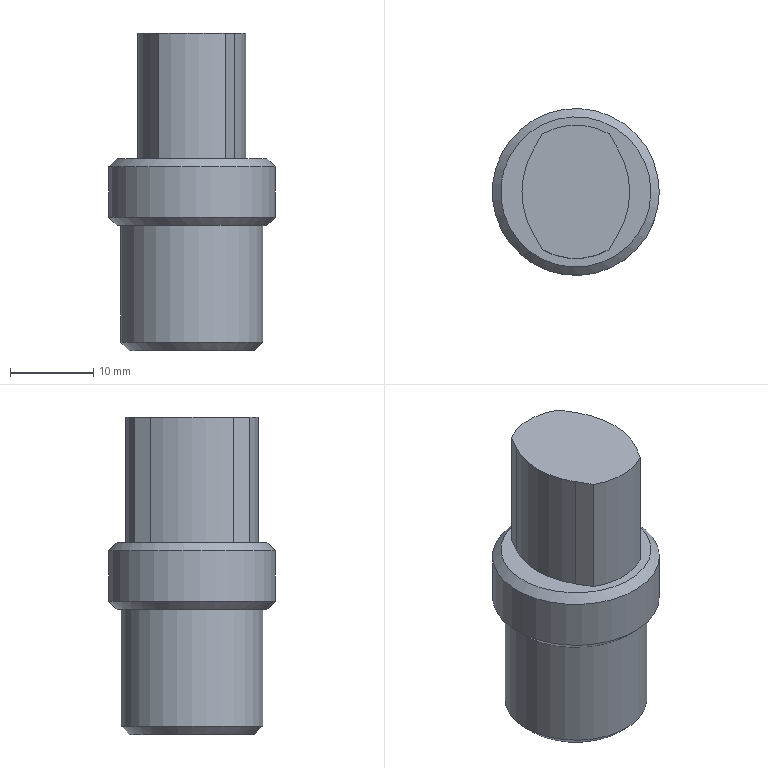Part | NX | features DATUM_CSYS 4, EXTRUDE 3, SKETCH 3, BLEND 1, CHAMFER 1 | 1 solid | 17 faces | box 20 x 20 x 38 mm | volume 8338 mm3 | plane 8 | cylinder 6 | cone 3 | commonest cylinder face diameters 20 x3 16 x2 17 x1
STEP:
#1=CARTESIAN_POINT('',(8.5,0.,1.));
#2=VERTEX_POINT('',#1);
#3=CARTESIAN_POINT('',(0.,0.,1.));
#4=DIRECTION('',(0.,0.,1.));
#5=DIRECTION('',(1.,0.,0.));
#6=AXIS2_PLACEMENT_3D('',#3,#4,#5);
#7=CIRCLE('',#6,8.5);
#8=EDGE_CURVE('',#2,#2,#7,.T.);
#9=ORIENTED_EDGE('',*,*,#8,.T.);
#10=EDGE_LOOP('',(#9));
#11=FACE_BOUND('',#10,.T.);
#12=CARTESIAN_POINT('',(8.5,0.,15.));
#13=VERTEX_POINT('',#12);
#14=CARTESIAN_POINT('',(0.,0.,15.));
#15=DIRECTION('',(0.,0.,1.));
#16=DIRECTION('',(1.,0.,0.));
#17=AXIS2_PLACEMENT_3D('',#14,#15,#16);
#18=CIRCLE('',#17,8.5);
#19=EDGE_CURVE('',#13,#13,#18,.T.);
#20=ORIENTED_EDGE('',*,*,#19,.F.);
#21=EDGE_LOOP('',(#20));
#22=FACE_BOUND('',#21,.T.);
#23=CARTESIAN_POINT('',(0.,0.,15.));
#24=DIRECTION('',(0.,0.,-1.));
#25=DIRECTION('',(-1.,0.,0.));
#26=AXIS2_PLACEMENT_3D('',#23,#24,#25);
#27=CYLINDRICAL_SURFACE('',#26,8.5);
#28=ADVANCED_FACE('',(#11,#22),#27,.T.);
#29=CARTESIAN_POINT('',(7.5,0.,0.));
#30=VERTEX_POINT('',#29);
#31=CARTESIAN_POINT('',(0.,0.,0.));
#32=DIRECTION('',(0.,0.,1.));
#33=DIRECTION('',(1.,0.,0.));
#34=AXIS2_PLACEMENT_3D('',#31,#32,#33);
#35=CIRCLE('',#34,7.5);
#36=EDGE_CURVE('',#30,#30,#35,.F.);
#37=ORIENTED_EDGE('',*,*,#36,.T.);
#38=EDGE_LOOP('',(#37));
#39=FACE_BOUND('',#38,.T.);
#40=CARTESIAN_POINT('',(0.,0.,0.));
#41=DIRECTION('',(0.,0.,1.));
#42=DIRECTION('',(1.,0.,0.));
#43=AXIS2_PLACEMENT_3D('',#40,#41,#42);
#44=PLANE('',#43);
#45=ADVANCED_FACE('',(#39),#44,.F.);
#46=CARTESIAN_POINT('',(10.,0.,22.));
#47=VERTEX_POINT('',#46);
#48=CARTESIAN_POINT('',(0.,0.,22.));
#49=DIRECTION('',(0.,0.,1.));
#50=DIRECTION('',(1.,0.,0.));
#51=AXIS2_PLACEMENT_3D('',#48,#49,#50);
#52=CIRCLE('',#51,10.);
#53=EDGE_CURVE('',#47,#47,#52,.F.);
#54=ORIENTED_EDGE('',*,*,#53,.T.);
#55=EDGE_LOOP('',(#54));
#56=FACE_BOUND('',#55,.T.);
#57=CARTESIAN_POINT('',(10.,0.,16.));
#58=VERTEX_POINT('',#57);
#59=CARTESIAN_POINT('',(0.,0.,16.));
#60=DIRECTION('',(0.,0.,1.));
#61=DIRECTION('',(1.,0.,0.));
#62=AXIS2_PLACEMENT_3D('',#59,#60,#61);
#63=CIRCLE('',#62,10.);
#64=EDGE_CURVE('',#58,#58,#63,.T.);
#65=ORIENTED_EDGE('',*,*,#64,.T.);
#66=EDGE_LOOP('',(#65));
#67=FACE_BOUND('',#66,.T.);
#68=CARTESIAN_POINT('',(0.,0.,23.));
#69=DIRECTION('',(0.,0.,-1.));
#70=DIRECTION('',(-1.,0.,0.));
#71=AXIS2_PLACEMENT_3D('',#68,#69,#70);
#72=CYLINDRICAL_SURFACE('',#71,10.);
#73=ADVANCED_FACE('',(#56,#67),#72,.T.);
#74=CARTESIAN_POINT('',(9.,0.,23.));
#75=VERTEX_POINT('',#74);
#76=CARTESIAN_POINT('',(0.,0.,23.));
#77=DIRECTION('',(0.,0.,1.));
#78=DIRECTION('',(1.,0.,0.));
#79=AXIS2_PLACEMENT_3D('',#76,#77,#78);
#80=CIRCLE('',#79,9.);
#81=EDGE_CURVE('',#75,#75,#80,.T.);
#82=ORIENTED_EDGE('',*,*,#81,.T.);
#83=EDGE_LOOP('',(#82));
#84=FACE_BOUND('',#83,.T.);
#85=CARTESIAN_POINT('',(5.113,5.,23.));
#86=VERTEX_POINT('',#85);
#87=CARTESIAN_POINT('',(4.,6.928,23.));
#88=VERTEX_POINT('',#87);
#89=CARTESIAN_POINT('',(8.,0.,23.));
#90=DIRECTION('',(-0.5,0.866,0.));
#91=VECTOR('',#90,1000.);
#92=LINE('',#89,#91);
#93=EDGE_CURVE('',#86,#88,#92,.T.);
#94=ORIENTED_EDGE('',*,*,#93,.F.);
#95=CARTESIAN_POINT('',(5.113,-5.,23.));
#96=VERTEX_POINT('',#95);
#97=CARTESIAN_POINT('',(-3.547,0.,23.));
#98=DIRECTION('',(0.,0.,1.));
#99=DIRECTION('',(1.,0.,0.));
#100=AXIS2_PLACEMENT_3D('',#97,#98,#99);
#101=CIRCLE('',#100,10.);
#102=EDGE_CURVE('',#86,#96,#101,.F.);
#103=ORIENTED_EDGE('',*,*,#102,.T.);
#104=CARTESIAN_POINT('',(4.,-6.928,23.));
#105=VERTEX_POINT('',#104);
#106=CARTESIAN_POINT('',(4.,-6.928,23.));
#107=DIRECTION('',(0.5,0.866,0.));
#108=VECTOR('',#107,1000.);
#109=LINE('',#106,#108);
#110=EDGE_CURVE('',#105,#96,#109,.T.);
#111=ORIENTED_EDGE('',*,*,#110,.F.);
#112=CARTESIAN_POINT('',(-4.,-6.928,23.));
#113=VERTEX_POINT('',#112);
#114=CARTESIAN_POINT('',(0.,0.,23.));
#115=DIRECTION('',(0.,0.,1.));
#116=DIRECTION('',(1.,0.,0.));
#117=AXIS2_PLACEMENT_3D('',#114,#115,#116);
#118=CIRCLE('',#117,8.);
#119=EDGE_CURVE('',#113,#105,#118,.T.);
#120=ORIENTED_EDGE('',*,*,#119,.F.);
#121=CARTESIAN_POINT('',(-5.113,-5.,23.));
#122=VERTEX_POINT('',#121);
#123=CARTESIAN_POINT('',(-8.,0.,23.));
#124=DIRECTION('',(0.5,-0.866,0.));
#125=VECTOR('',#124,1000.);
#126=LINE('',#123,#125);
#127=EDGE_CURVE('',#122,#113,#126,.T.);
#128=ORIENTED_EDGE('',*,*,#127,.F.);
#129=CARTESIAN_POINT('',(-5.113,5.,23.));
#130=VERTEX_POINT('',#129);
#131=CARTESIAN_POINT('',(3.547,0.,23.));
#132=DIRECTION('',(0.,0.,1.));
#133=DIRECTION('',(1.,0.,0.));
#134=AXIS2_PLACEMENT_3D('',#131,#132,#133);
#135=CIRCLE('',#134,10.);
#136=EDGE_CURVE('',#122,#130,#135,.F.);
#137=ORIENTED_EDGE('',*,*,#136,.T.);
#138=CARTESIAN_POINT('',(-4.,6.928,23.));
#139=VERTEX_POINT('',#138);
#140=CARTESIAN_POINT('',(-4.,6.928,23.));
#141=DIRECTION('',(-0.5,-0.866,0.));
#142=VECTOR('',#141,1000.);
#143=LINE('',#140,#142);
#144=EDGE_CURVE('',#139,#130,#143,.T.);
#145=ORIENTED_EDGE('',*,*,#144,.F.);
#146=CARTESIAN_POINT('',(0.,0.,23.));
#147=DIRECTION('',(0.,0.,1.));
#148=DIRECTION('',(1.,0.,0.));
#149=AXIS2_PLACEMENT_3D('',#146,#147,#148);
#150=CIRCLE('',#149,8.);
#151=EDGE_CURVE('',#88,#139,#150,.T.);
#152=ORIENTED_EDGE('',*,*,#151,.F.);
#153=EDGE_LOOP('',(#94,#103,#111,#120,#128,#137,#145,#152));
#154=FACE_BOUND('',#153,.T.);
#155=CARTESIAN_POINT('',(0.,0.,23.));
#156=DIRECTION('',(0.,0.,1.));
#157=DIRECTION('',(1.,0.,0.));
#158=AXIS2_PLACEMENT_3D('',#155,#156,#157);
#159=PLANE('',#158);
#160=ADVANCED_FACE('',(#84,#154),#159,.T.);
#161=CARTESIAN_POINT('',(9.,0.,15.));
#162=VERTEX_POINT('',#161);
#163=CARTESIAN_POINT('',(0.,0.,15.));
#164=DIRECTION('',(0.,0.,1.));
#165=DIRECTION('',(1.,0.,0.));
#166=AXIS2_PLACEMENT_3D('',#163,#164,#165);
#167=CIRCLE('',#166,9.);
#168=EDGE_CURVE('',#162,#162,#167,.F.);
#169=ORIENTED_EDGE('',*,*,#168,.T.);
#170=EDGE_LOOP('',(#169));
#171=FACE_BOUND('',#170,.T.);
#172=ORIENTED_EDGE('',*,*,#19,.T.);
#173=EDGE_LOOP('',(#172));
#174=FACE_BOUND('',#173,.T.);
#175=CARTESIAN_POINT('',(0.,0.,15.));
#176=DIRECTION('',(0.,0.,1.));
#177=DIRECTION('',(1.,0.,0.));
#178=AXIS2_PLACEMENT_3D('',#175,#176,#177);
#179=PLANE('',#178);
#180=ADVANCED_FACE('',(#171,#174),#179,.F.);
#181=CARTESIAN_POINT('',(5.113,5.,38.));
#182=VERTEX_POINT('',#181);
#183=CARTESIAN_POINT('',(4.,6.928,38.));
#184=VERTEX_POINT('',#183);
#185=CARTESIAN_POINT('',(8.,0.,38.));
#186=DIRECTION('',(-0.5,0.866,0.));
#187=VECTOR('',#186,1000.);
#188=LINE('',#185,#187);
#189=EDGE_CURVE('',#182,#184,#188,.T.);
#190=ORIENTED_EDGE('',*,*,#189,.F.);
#191=CARTESIAN_POINT('',(5.113,5.,38.));
#192=DIRECTION('',(0.,0.,-1.));
#193=VECTOR('',#192,1000.);
#194=LINE('',#191,#193);
#195=EDGE_CURVE('',#182,#86,#194,.T.);
#196=ORIENTED_EDGE('',*,*,#195,.T.);
#197=ORIENTED_EDGE('',*,*,#93,.T.);
#198=CARTESIAN_POINT('',(4.,6.928,38.));
#199=DIRECTION('',(0.,0.,-1.));
#200=VECTOR('',#199,1000.);
#201=LINE('',#198,#200);
#202=EDGE_CURVE('',#184,#88,#201,.T.);
#203=ORIENTED_EDGE('',*,*,#202,.F.);
#204=EDGE_LOOP('',(#190,#196,#197,#203));
#205=FACE_BOUND('',#204,.T.);
#206=CARTESIAN_POINT('',(8.,0.,38.));
#207=DIRECTION('',(-0.866,-0.5,0.));
#208=DIRECTION('',(0.5,-0.866,0.));
#209=AXIS2_PLACEMENT_3D('',#206,#207,#208);
#210=PLANE('',#209);
#211=ADVANCED_FACE('',(#205),#210,.F.);
#212=ORIENTED_EDGE('',*,*,#151,.T.);
#213=CARTESIAN_POINT('',(-4.,6.928,38.));
#214=VERTEX_POINT('',#213);
#215=CARTESIAN_POINT('',(-4.,6.928,38.));
#216=DIRECTION('',(0.,0.,-1.));
#217=VECTOR('',#216,1000.);
#218=LINE('',#215,#217);
#219=EDGE_CURVE('',#214,#139,#218,.T.);
#220=ORIENTED_EDGE('',*,*,#219,.F.);
#221=CARTESIAN_POINT('',(0.,0.,38.));
#222=DIRECTION('',(0.,0.,1.));
#223=DIRECTION('',(1.,0.,0.));
#224=AXIS2_PLACEMENT_3D('',#221,#222,#223);
#225=CIRCLE('',#224,8.);
#226=EDGE_CURVE('',#184,#214,#225,.T.);
#227=ORIENTED_EDGE('',*,*,#226,.F.);
#228=ORIENTED_EDGE('',*,*,#202,.T.);
#229=EDGE_LOOP('',(#212,#220,#227,#228));
#230=FACE_BOUND('',#229,.T.);
#231=CARTESIAN_POINT('',(0.,0.,38.));
#232=DIRECTION('',(0.,0.,-1.));
#233=DIRECTION('',(-1.,0.,0.));
#234=AXIS2_PLACEMENT_3D('',#231,#232,#233);
#235=CYLINDRICAL_SURFACE('',#234,8.);
#236=ADVANCED_FACE('',(#230),#235,.T.);
#237=ORIENTED_EDGE('',*,*,#144,.T.);
#238=CARTESIAN_POINT('',(-5.113,5.,38.));
#239=VERTEX_POINT('',#238);
#240=CARTESIAN_POINT('',(-5.113,5.,38.));
#241=DIRECTION('',(0.,0.,-1.));
#242=VECTOR('',#241,1000.);
#243=LINE('',#240,#242);
#244=EDGE_CURVE('',#130,#239,#243,.F.);
#245=ORIENTED_EDGE('',*,*,#244,.T.);
#246=CARTESIAN_POINT('',(-4.,6.928,38.));
#247=DIRECTION('',(-0.5,-0.866,0.));
#248=VECTOR('',#247,1000.);
#249=LINE('',#246,#248);
#250=EDGE_CURVE('',#214,#239,#249,.T.);
#251=ORIENTED_EDGE('',*,*,#250,.F.);
#252=ORIENTED_EDGE('',*,*,#219,.T.);
#253=EDGE_LOOP('',(#237,#245,#251,#252));
#254=FACE_BOUND('',#253,.T.);
#255=CARTESIAN_POINT('',(-4.,6.928,38.));
#256=DIRECTION('',(0.866,-0.5,0.));
#257=DIRECTION('',(0.5,0.866,0.));
#258=AXIS2_PLACEMENT_3D('',#255,#256,#257);
#259=PLANE('',#258);
#260=ADVANCED_FACE('',(#254),#259,.F.);
#261=CARTESIAN_POINT('',(-5.113,-5.,38.));
#262=VERTEX_POINT('',#261);
#263=CARTESIAN_POINT('',(-4.,-6.928,38.));
#264=VERTEX_POINT('',#263);
#265=CARTESIAN_POINT('',(-8.,0.,38.));
#266=DIRECTION('',(0.5,-0.866,0.));
#267=VECTOR('',#266,1000.);
#268=LINE('',#265,#267);
#269=EDGE_CURVE('',#262,#264,#268,.T.);
#270=ORIENTED_EDGE('',*,*,#269,.F.);
#271=CARTESIAN_POINT('',(-5.113,-5.,38.));
#272=DIRECTION('',(0.,0.,-1.));
#273=VECTOR('',#272,1000.);
#274=LINE('',#271,#273);
#275=EDGE_CURVE('',#262,#122,#274,.T.);
#276=ORIENTED_EDGE('',*,*,#275,.T.);
#277=ORIENTED_EDGE('',*,*,#127,.T.);
#278=CARTESIAN_POINT('',(-4.,-6.928,38.));
#279=DIRECTION('',(0.,0.,-1.));
#280=VECTOR('',#279,1000.);
#281=LINE('',#278,#280);
#282=EDGE_CURVE('',#264,#113,#281,.T.);
#283=ORIENTED_EDGE('',*,*,#282,.F.);
#284=EDGE_LOOP('',(#270,#276,#277,#283));
#285=FACE_BOUND('',#284,.T.);
#286=CARTESIAN_POINT('',(-8.,0.,38.));
#287=DIRECTION('',(0.866,0.5,0.));
#288=DIRECTION('',(-0.5,0.866,0.));
#289=AXIS2_PLACEMENT_3D('',#286,#287,#288);
#290=PLANE('',#289);
#291=ADVANCED_FACE('',(#285),#290,.F.);
#292=ORIENTED_EDGE('',*,*,#119,.T.);
#293=CARTESIAN_POINT('',(4.,-6.928,38.));
#294=VERTEX_POINT('',#293);
#295=CARTESIAN_POINT('',(4.,-6.928,38.));
#296=DIRECTION('',(0.,0.,-1.));
#297=VECTOR('',#296,1000.);
#298=LINE('',#295,#297);
#299=EDGE_CURVE('',#294,#105,#298,.T.);
#300=ORIENTED_EDGE('',*,*,#299,.F.);
#301=CARTESIAN_POINT('',(0.,0.,38.));
#302=DIRECTION('',(0.,0.,1.));
#303=DIRECTION('',(1.,0.,0.));
#304=AXIS2_PLACEMENT_3D('',#301,#302,#303);
#305=CIRCLE('',#304,8.);
#306=EDGE_CURVE('',#264,#294,#305,.T.);
#307=ORIENTED_EDGE('',*,*,#306,.F.);
#308=ORIENTED_EDGE('',*,*,#282,.T.);
#309=EDGE_LOOP('',(#292,#300,#307,#308));
#310=FACE_BOUND('',#309,.T.);
#311=CARTESIAN_POINT('',(0.,0.,38.));
#312=DIRECTION('',(0.,0.,-1.));
#313=DIRECTION('',(-1.,0.,0.));
#314=AXIS2_PLACEMENT_3D('',#311,#312,#313);
#315=CYLINDRICAL_SURFACE('',#314,8.);
#316=ADVANCED_FACE('',(#310),#315,.T.);
#317=ORIENTED_EDGE('',*,*,#110,.T.);
#318=CARTESIAN_POINT('',(5.113,-5.,38.));
#319=VERTEX_POINT('',#318);
#320=CARTESIAN_POINT('',(5.113,-5.,38.));
#321=DIRECTION('',(0.,0.,-1.));
#322=VECTOR('',#321,1000.);
#323=LINE('',#320,#322);
#324=EDGE_CURVE('',#96,#319,#323,.F.);
#325=ORIENTED_EDGE('',*,*,#324,.T.);
#326=CARTESIAN_POINT('',(4.,-6.928,38.));
#327=DIRECTION('',(0.5,0.866,0.));
#328=VECTOR('',#327,1000.);
#329=LINE('',#326,#328);
#330=EDGE_CURVE('',#294,#319,#329,.T.);
#331=ORIENTED_EDGE('',*,*,#330,.F.);
#332=ORIENTED_EDGE('',*,*,#299,.T.);
#333=EDGE_LOOP('',(#317,#325,#331,#332));
#334=FACE_BOUND('',#333,.T.);
#335=CARTESIAN_POINT('',(4.,-6.928,38.));
#336=DIRECTION('',(-0.866,0.5,0.));
#337=DIRECTION('',(-0.5,-0.866,0.));
#338=AXIS2_PLACEMENT_3D('',#335,#336,#337);
#339=PLANE('',#338);
#340=ADVANCED_FACE('',(#334),#339,.F.);
#341=ORIENTED_EDGE('',*,*,#330,.T.);
#342=CARTESIAN_POINT('',(-3.547,0.,38.));
#343=DIRECTION('',(0.,0.,1.));
#344=DIRECTION('',(1.,0.,0.));
#345=AXIS2_PLACEMENT_3D('',#342,#343,#344);
#346=CIRCLE('',#345,10.);
#347=EDGE_CURVE('',#319,#182,#346,.T.);
#348=ORIENTED_EDGE('',*,*,#347,.T.);
#349=ORIENTED_EDGE('',*,*,#189,.T.);
#350=ORIENTED_EDGE('',*,*,#226,.T.);
#351=ORIENTED_EDGE('',*,*,#250,.T.);
#352=CARTESIAN_POINT('',(3.547,0.,38.));
#353=DIRECTION('',(0.,0.,1.));
#354=DIRECTION('',(1.,0.,0.));
#355=AXIS2_PLACEMENT_3D('',#352,#353,#354);
#356=CIRCLE('',#355,10.);
#357=EDGE_CURVE('',#239,#262,#356,.T.);
#358=ORIENTED_EDGE('',*,*,#357,.T.);
#359=ORIENTED_EDGE('',*,*,#269,.T.);
#360=ORIENTED_EDGE('',*,*,#306,.T.);
#361=EDGE_LOOP('',(#341,#348,#349,#350,#351,#358,#359,#360));
#362=FACE_BOUND('',#361,.T.);
#363=CARTESIAN_POINT('',(0.,0.,38.));
#364=DIRECTION('',(0.,0.,1.));
#365=DIRECTION('',(1.,0.,0.));
#366=AXIS2_PLACEMENT_3D('',#363,#364,#365);
#367=PLANE('',#366);
#368=ADVANCED_FACE('',(#362),#367,.T.);
#369=ORIENTED_EDGE('',*,*,#53,.F.);
#370=EDGE_LOOP('',(#369));
#371=FACE_BOUND('',#370,.T.);
#372=ORIENTED_EDGE('',*,*,#81,.F.);
#373=EDGE_LOOP('',(#372));
#374=FACE_BOUND('',#373,.T.);
#375=CARTESIAN_POINT('',(0.,0.,23.));
#376=DIRECTION('',(0.,0.,-1.));
#377=DIRECTION('',(-1.,0.,0.));
#378=AXIS2_PLACEMENT_3D('',#375,#376,#377);
#379=CONICAL_SURFACE('',#378,9.,0.7854);
#380=ADVANCED_FACE('',(#371,#374),#379,.T.);
#381=ORIENTED_EDGE('',*,*,#36,.F.);
#382=EDGE_LOOP('',(#381));
#383=FACE_BOUND('',#382,.T.);
#384=ORIENTED_EDGE('',*,*,#8,.F.);
#385=EDGE_LOOP('',(#384));
#386=FACE_BOUND('',#385,.T.);
#387=CARTESIAN_POINT('',(0.,0.,1.));
#388=DIRECTION('',(0.,0.,1.));
#389=DIRECTION('',(1.,0.,0.));
#390=AXIS2_PLACEMENT_3D('',#387,#388,#389);
#391=CONICAL_SURFACE('',#390,8.5,0.7854);
#392=ADVANCED_FACE('',(#383,#386),#391,.T.);
#393=ORIENTED_EDGE('',*,*,#168,.F.);
#394=EDGE_LOOP('',(#393));
#395=FACE_BOUND('',#394,.T.);
#396=ORIENTED_EDGE('',*,*,#64,.F.);
#397=EDGE_LOOP('',(#396));
#398=FACE_BOUND('',#397,.T.);
#399=CARTESIAN_POINT('',(0.,0.,16.));
#400=DIRECTION('',(0.,0.,1.));
#401=DIRECTION('',(1.,0.,0.));
#402=AXIS2_PLACEMENT_3D('',#399,#400,#401);
#403=CONICAL_SURFACE('',#402,10.,0.7854);
#404=ADVANCED_FACE('',(#395,#398),#403,.T.);
#405=ORIENTED_EDGE('',*,*,#347,.F.);
#406=ORIENTED_EDGE('',*,*,#324,.F.);
#407=ORIENTED_EDGE('',*,*,#102,.F.);
#408=ORIENTED_EDGE('',*,*,#195,.F.);
#409=EDGE_LOOP('',(#405,#406,#407,#408));
#410=FACE_BOUND('',#409,.T.);
#411=CARTESIAN_POINT('',(-3.547,0.,38.));
#412=DIRECTION('',(0.,0.,-1.));
#413=DIRECTION('',(-1.,0.,0.));
#414=AXIS2_PLACEMENT_3D('',#411,#412,#413);
#415=CYLINDRICAL_SURFACE('',#414,10.);
#416=ADVANCED_FACE('',(#410),#415,.T.);
#417=ORIENTED_EDGE('',*,*,#357,.F.);
#418=ORIENTED_EDGE('',*,*,#244,.F.);
#419=ORIENTED_EDGE('',*,*,#136,.F.);
#420=ORIENTED_EDGE('',*,*,#275,.F.);
#421=EDGE_LOOP('',(#417,#418,#419,#420));
#422=FACE_BOUND('',#421,.T.);
#423=CARTESIAN_POINT('',(3.547,0.,38.));
#424=DIRECTION('',(0.,0.,-1.));
#425=DIRECTION('',(-1.,0.,0.));
#426=AXIS2_PLACEMENT_3D('',#423,#424,#425);
#427=CYLINDRICAL_SURFACE('',#426,10.);
#428=ADVANCED_FACE('',(#422),#427,.T.);
#429=CLOSED_SHELL('',(#28,#45,#73,#160,#180,#211,#236,#260,#291,#316,#340,#368,#380,#392,#404,#416,#428));
#430=MANIFOLD_SOLID_BREP('',#429);
#431=(LENGTH_UNIT()NAMED_UNIT(*)SI_UNIT(.MILLI.,.METRE.));
#432=UNCERTAINTY_MEASURE_WITH_UNIT(LENGTH_MEASURE(0.00001),#431,'','');
#433=(NAMED_UNIT(*)PLANE_ANGLE_UNIT()SI_UNIT($,.RADIAN.));
#434=(NAMED_UNIT(*)SI_UNIT($,.STERADIAN.)SOLID_ANGLE_UNIT());
#435=(GEOMETRIC_REPRESENTATION_CONTEXT(3)GLOBAL_UNCERTAINTY_ASSIGNED_CONTEXT((#432))GLOBAL_UNIT_ASSIGNED_CONTEXT((#431,#433,#434))REPRESENTATION_CONTEXT('',''));
#436=ADVANCED_BREP_SHAPE_REPRESENTATION('',(#430),#435);